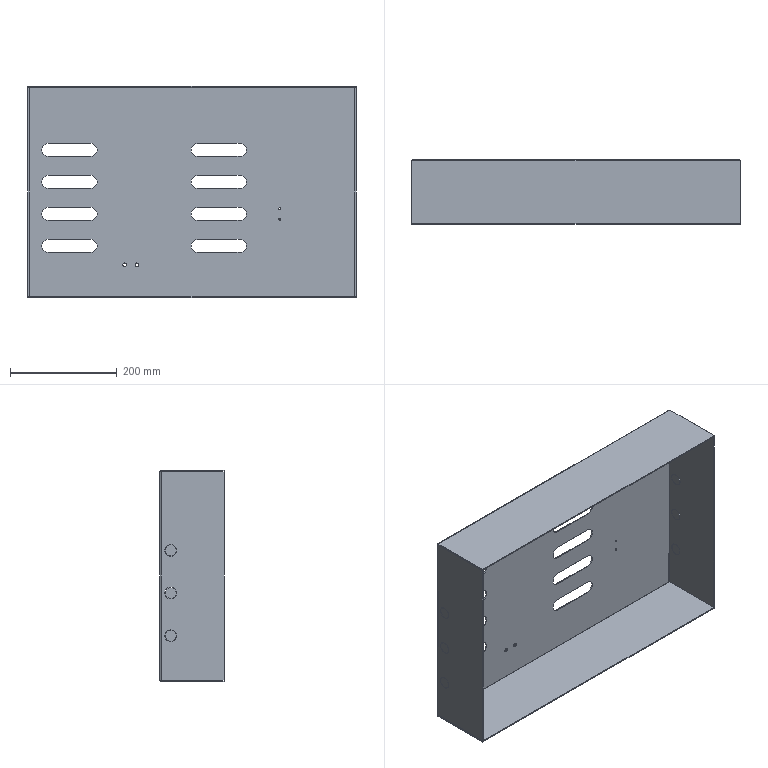Part | SolidWorks | features BaseBody 1 | 1 solid | 134 faces | box 615 x 120 x 396 mm | volume 920758 mm3 | plane 78 | cylinder 56 | commonest cylinder face diameters 24 x16 21 x12 22 x12 0.4 x4 3.3 x4 4.4 x4